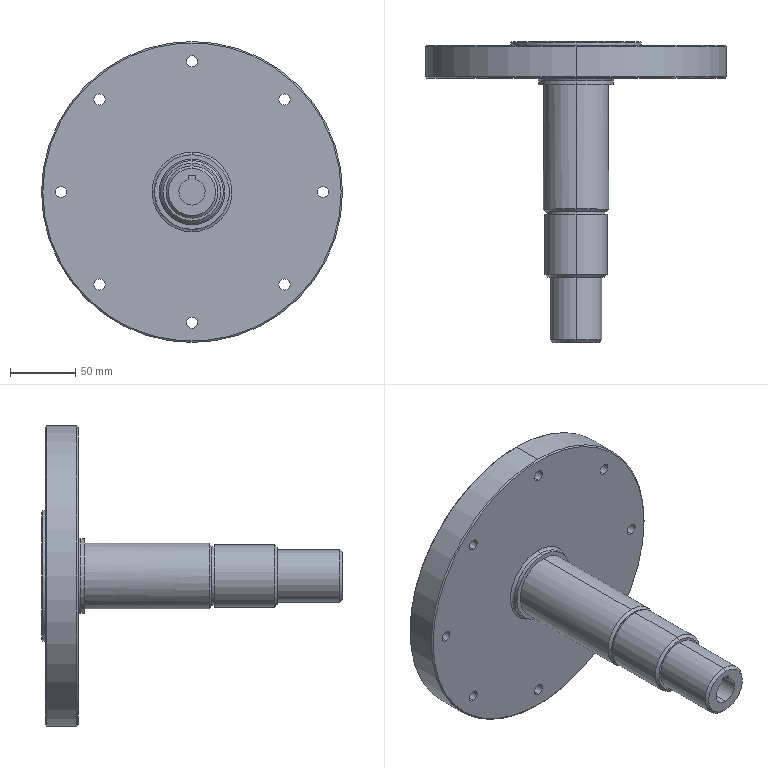Part | STEP file | BB013A02M-04-02A | 1 solid | 58 faces | box 230 x 230 x 230 mm | volume 1390467 mm3 | cylinder 32 | cone 12 | plane 12 | spline 2 | commonest cylinder face diameters 8.5 x16 20 x2 40 x2 45 x2 48 x2 50 x2